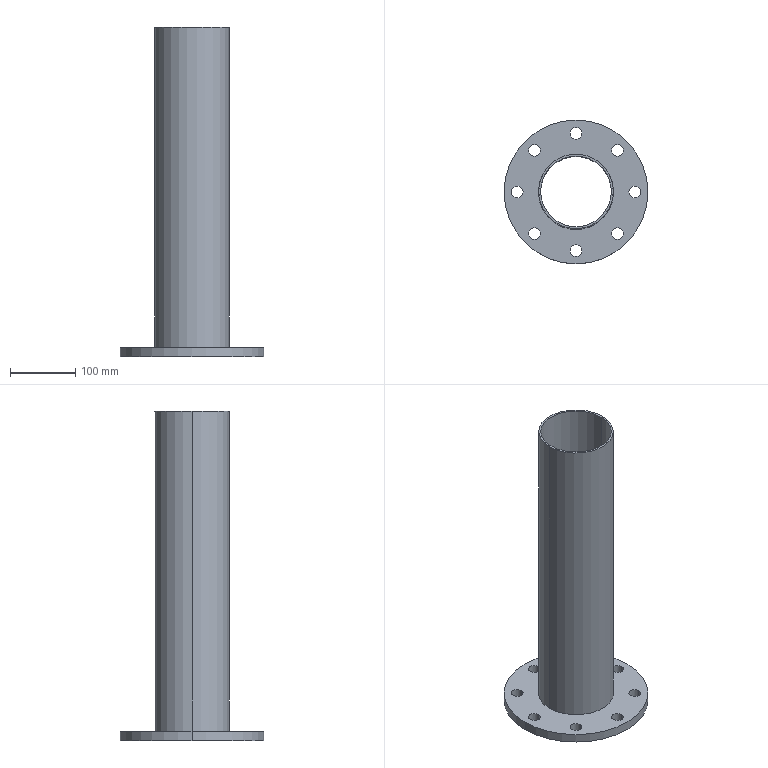Part | SolidWorks | features Extrusion 1, ICE 1 | 2 solids | 28 faces | box 220 x 220 x 504 mm | volume 882758 mm3 | cylinder 24 | plane 4 | commonest cylinder face diameters 18 x16 108.3 x2 114.3 x2 115 x2 220 x2
STEP:
#1=CARTESIAN_POINT('',(-72.64,63.64,14.));
#2=VERTEX_POINT('',#1);
#3=CARTESIAN_POINT('',(-54.64,63.64,14.));
#4=VERTEX_POINT('',#3);
#5=CARTESIAN_POINT('',(-63.64,63.64,14.));
#6=DIRECTION('',(0.,0.,1.));
#7=DIRECTION('',(1.,0.,0.));
#8=AXIS2_PLACEMENT_3D('',#5,#6,#7);
#9=CIRCLE('',#8,9.);
#10=EDGE_CURVE('',#2,#4,#9,.T.);
#11=ORIENTED_EDGE('',*,*,#10,.T.);
#12=CARTESIAN_POINT('',(-54.64,63.64,0.));
#13=VERTEX_POINT('',#12);
#14=CARTESIAN_POINT('',(-54.64,63.64,14.));
#15=DIRECTION('',(0.,0.,-1.));
#16=VECTOR('',#15,1000.);
#17=LINE('',#14,#16);
#18=EDGE_CURVE('',#4,#13,#17,.T.);
#19=ORIENTED_EDGE('',*,*,#18,.T.);
#20=CARTESIAN_POINT('',(-72.64,63.64,0.));
#21=VERTEX_POINT('',#20);
#22=CARTESIAN_POINT('',(-63.64,63.64,0.));
#23=DIRECTION('',(0.,0.,1.));
#24=DIRECTION('',(1.,0.,0.));
#25=AXIS2_PLACEMENT_3D('',#22,#23,#24);
#26=CIRCLE('',#25,9.);
#27=EDGE_CURVE('',#21,#13,#26,.T.);
#28=ORIENTED_EDGE('',*,*,#27,.F.);
#29=CARTESIAN_POINT('',(-72.64,63.64,14.));
#30=DIRECTION('',(0.,0.,-1.));
#31=VECTOR('',#30,1000.);
#32=LINE('',#29,#31);
#33=EDGE_CURVE('',#2,#21,#32,.T.);
#34=ORIENTED_EDGE('',*,*,#33,.F.);
#35=EDGE_LOOP('',(#11,#19,#28,#34));
#36=FACE_OUTER_BOUND('',#35,.T.);
#37=CARTESIAN_POINT('',(-63.64,63.64,14.));
#38=DIRECTION('',(0.,0.,-1.));
#39=DIRECTION('',(-1.,0.,0.));
#40=AXIS2_PLACEMENT_3D('',#37,#38,#39);
#41=CYLINDRICAL_SURFACE('',#40,9.);
#42=ADVANCED_FACE('',(#36),#41,.F.);
#43=CARTESIAN_POINT('',(-99.,0.,14.));
#44=VERTEX_POINT('',#43);
#45=CARTESIAN_POINT('',(-81.,0.,14.));
#46=VERTEX_POINT('',#45);
#47=CARTESIAN_POINT('',(-90.,0.,14.));
#48=DIRECTION('',(0.,0.,1.));
#49=DIRECTION('',(1.,0.,0.));
#50=AXIS2_PLACEMENT_3D('',#47,#48,#49);
#51=CIRCLE('',#50,9.);
#52=EDGE_CURVE('',#44,#46,#51,.T.);
#53=ORIENTED_EDGE('',*,*,#52,.T.);
#54=CARTESIAN_POINT('',(-81.,0.,0.));
#55=VERTEX_POINT('',#54);
#56=CARTESIAN_POINT('',(-81.,0.,14.));
#57=DIRECTION('',(0.,0.,-1.));
#58=VECTOR('',#57,1000.);
#59=LINE('',#56,#58);
#60=EDGE_CURVE('',#46,#55,#59,.T.);
#61=ORIENTED_EDGE('',*,*,#60,.T.);
#62=CARTESIAN_POINT('',(-99.,0.,0.));
#63=VERTEX_POINT('',#62);
#64=CARTESIAN_POINT('',(-90.,0.,0.));
#65=DIRECTION('',(0.,0.,1.));
#66=DIRECTION('',(1.,0.,0.));
#67=AXIS2_PLACEMENT_3D('',#64,#65,#66);
#68=CIRCLE('',#67,9.);
#69=EDGE_CURVE('',#63,#55,#68,.T.);
#70=ORIENTED_EDGE('',*,*,#69,.F.);
#71=CARTESIAN_POINT('',(-99.,0.,14.));
#72=DIRECTION('',(0.,0.,-1.));
#73=VECTOR('',#72,1000.);
#74=LINE('',#71,#73);
#75=EDGE_CURVE('',#44,#63,#74,.T.);
#76=ORIENTED_EDGE('',*,*,#75,.F.);
#77=EDGE_LOOP('',(#53,#61,#70,#76));
#78=FACE_OUTER_BOUND('',#77,.T.);
#79=CARTESIAN_POINT('',(-90.,0.,14.));
#80=DIRECTION('',(0.,0.,-1.));
#81=DIRECTION('',(-1.,0.,0.));
#82=AXIS2_PLACEMENT_3D('',#79,#80,#81);
#83=CYLINDRICAL_SURFACE('',#82,9.);
#84=ADVANCED_FACE('',(#78),#83,.F.);
#85=CARTESIAN_POINT('',(-72.64,-63.64,14.));
#86=VERTEX_POINT('',#85);
#87=CARTESIAN_POINT('',(-54.64,-63.64,14.));
#88=VERTEX_POINT('',#87);
#89=CARTESIAN_POINT('',(-63.64,-63.64,14.));
#90=DIRECTION('',(0.,0.,1.));
#91=DIRECTION('',(1.,0.,0.));
#92=AXIS2_PLACEMENT_3D('',#89,#90,#91);
#93=CIRCLE('',#92,9.);
#94=EDGE_CURVE('',#86,#88,#93,.T.);
#95=ORIENTED_EDGE('',*,*,#94,.T.);
#96=CARTESIAN_POINT('',(-54.64,-63.64,0.));
#97=VERTEX_POINT('',#96);
#98=CARTESIAN_POINT('',(-54.64,-63.64,14.));
#99=DIRECTION('',(0.,0.,-1.));
#100=VECTOR('',#99,1000.);
#101=LINE('',#98,#100);
#102=EDGE_CURVE('',#88,#97,#101,.T.);
#103=ORIENTED_EDGE('',*,*,#102,.T.);
#104=CARTESIAN_POINT('',(-72.64,-63.64,0.));
#105=VERTEX_POINT('',#104);
#106=CARTESIAN_POINT('',(-63.64,-63.64,0.));
#107=DIRECTION('',(0.,0.,1.));
#108=DIRECTION('',(1.,0.,0.));
#109=AXIS2_PLACEMENT_3D('',#106,#107,#108);
#110=CIRCLE('',#109,9.);
#111=EDGE_CURVE('',#105,#97,#110,.T.);
#112=ORIENTED_EDGE('',*,*,#111,.F.);
#113=CARTESIAN_POINT('',(-72.64,-63.64,14.));
#114=DIRECTION('',(0.,0.,-1.));
#115=VECTOR('',#114,1000.);
#116=LINE('',#113,#115);
#117=EDGE_CURVE('',#86,#105,#116,.T.);
#118=ORIENTED_EDGE('',*,*,#117,.F.);
#119=EDGE_LOOP('',(#95,#103,#112,#118));
#120=FACE_OUTER_BOUND('',#119,.T.);
#121=CARTESIAN_POINT('',(-63.64,-63.64,14.));
#122=DIRECTION('',(0.,0.,-1.));
#123=DIRECTION('',(-1.,0.,0.));
#124=AXIS2_PLACEMENT_3D('',#121,#122,#123);
#125=CYLINDRICAL_SURFACE('',#124,9.);
#126=ADVANCED_FACE('',(#120),#125,.F.);
#127=CARTESIAN_POINT('',(-9.,-90.,14.));
#128=VERTEX_POINT('',#127);
#129=CARTESIAN_POINT('',(9.,-90.,14.));
#130=VERTEX_POINT('',#129);
#131=CARTESIAN_POINT('',(0.,-90.,14.));
#132=DIRECTION('',(0.,0.,1.));
#133=DIRECTION('',(1.,0.,0.));
#134=AXIS2_PLACEMENT_3D('',#131,#132,#133);
#135=CIRCLE('',#134,9.);
#136=EDGE_CURVE('',#128,#130,#135,.T.);
#137=ORIENTED_EDGE('',*,*,#136,.T.);
#138=CARTESIAN_POINT('',(9.,-90.,0.));
#139=VERTEX_POINT('',#138);
#140=CARTESIAN_POINT('',(9.,-90.,14.));
#141=DIRECTION('',(0.,0.,-1.));
#142=VECTOR('',#141,1000.);
#143=LINE('',#140,#142);
#144=EDGE_CURVE('',#130,#139,#143,.T.);
#145=ORIENTED_EDGE('',*,*,#144,.T.);
#146=CARTESIAN_POINT('',(-9.,-90.,0.));
#147=VERTEX_POINT('',#146);
#148=CARTESIAN_POINT('',(0.,-90.,0.));
#149=DIRECTION('',(0.,0.,1.));
#150=DIRECTION('',(1.,0.,0.));
#151=AXIS2_PLACEMENT_3D('',#148,#149,#150);
#152=CIRCLE('',#151,9.);
#153=EDGE_CURVE('',#147,#139,#152,.T.);
#154=ORIENTED_EDGE('',*,*,#153,.F.);
#155=CARTESIAN_POINT('',(-9.,-90.,14.));
#156=DIRECTION('',(0.,0.,-1.));
#157=VECTOR('',#156,1000.);
#158=LINE('',#155,#157);
#159=EDGE_CURVE('',#128,#147,#158,.T.);
#160=ORIENTED_EDGE('',*,*,#159,.F.);
#161=EDGE_LOOP('',(#137,#145,#154,#160));
#162=FACE_OUTER_BOUND('',#161,.T.);
#163=CARTESIAN_POINT('',(0.,-90.,14.));
#164=DIRECTION('',(0.,0.,-1.));
#165=DIRECTION('',(-1.,0.,0.));
#166=AXIS2_PLACEMENT_3D('',#163,#164,#165);
#167=CYLINDRICAL_SURFACE('',#166,9.);
#168=ADVANCED_FACE('',(#162),#167,.F.);
#169=CARTESIAN_POINT('',(54.64,-63.64,14.));
#170=VERTEX_POINT('',#169);
#171=CARTESIAN_POINT('',(72.64,-63.64,14.));
#172=VERTEX_POINT('',#171);
#173=CARTESIAN_POINT('',(63.64,-63.64,14.));
#174=DIRECTION('',(0.,0.,1.));
#175=DIRECTION('',(1.,0.,0.));
#176=AXIS2_PLACEMENT_3D('',#173,#174,#175);
#177=CIRCLE('',#176,9.);
#178=EDGE_CURVE('',#170,#172,#177,.T.);
#179=ORIENTED_EDGE('',*,*,#178,.T.);
#180=CARTESIAN_POINT('',(72.64,-63.64,0.));
#181=VERTEX_POINT('',#180);
#182=CARTESIAN_POINT('',(72.64,-63.64,14.));
#183=DIRECTION('',(0.,0.,-1.));
#184=VECTOR('',#183,1000.);
#185=LINE('',#182,#184);
#186=EDGE_CURVE('',#172,#181,#185,.T.);
#187=ORIENTED_EDGE('',*,*,#186,.T.);
#188=CARTESIAN_POINT('',(54.64,-63.64,0.));
#189=VERTEX_POINT('',#188);
#190=CARTESIAN_POINT('',(63.64,-63.64,0.));
#191=DIRECTION('',(0.,0.,1.));
#192=DIRECTION('',(1.,0.,0.));
#193=AXIS2_PLACEMENT_3D('',#190,#191,#192);
#194=CIRCLE('',#193,9.);
#195=EDGE_CURVE('',#189,#181,#194,.T.);
#196=ORIENTED_EDGE('',*,*,#195,.F.);
#197=CARTESIAN_POINT('',(54.64,-63.64,14.));
#198=DIRECTION('',(0.,0.,-1.));
#199=VECTOR('',#198,1000.);
#200=LINE('',#197,#199);
#201=EDGE_CURVE('',#170,#189,#200,.T.);
#202=ORIENTED_EDGE('',*,*,#201,.F.);
#203=EDGE_LOOP('',(#179,#187,#196,#202));
#204=FACE_OUTER_BOUND('',#203,.T.);
#205=CARTESIAN_POINT('',(63.64,-63.64,14.));
#206=DIRECTION('',(0.,0.,-1.));
#207=DIRECTION('',(-1.,0.,0.));
#208=AXIS2_PLACEMENT_3D('',#205,#206,#207);
#209=CYLINDRICAL_SURFACE('',#208,9.);
#210=ADVANCED_FACE('',(#204),#209,.F.);
#211=CARTESIAN_POINT('',(81.,0.,14.));
#212=VERTEX_POINT('',#211);
#213=CARTESIAN_POINT('',(99.,0.,14.));
#214=VERTEX_POINT('',#213);
#215=CARTESIAN_POINT('',(90.,0.,14.));
#216=DIRECTION('',(0.,0.,1.));
#217=DIRECTION('',(1.,0.,0.));
#218=AXIS2_PLACEMENT_3D('',#215,#216,#217);
#219=CIRCLE('',#218,9.);
#220=EDGE_CURVE('',#212,#214,#219,.T.);
#221=ORIENTED_EDGE('',*,*,#220,.T.);
#222=CARTESIAN_POINT('',(99.,0.,0.));
#223=VERTEX_POINT('',#222);
#224=CARTESIAN_POINT('',(99.,0.,14.));
#225=DIRECTION('',(0.,0.,-1.));
#226=VECTOR('',#225,1000.);
#227=LINE('',#224,#226);
#228=EDGE_CURVE('',#214,#223,#227,.T.);
#229=ORIENTED_EDGE('',*,*,#228,.T.);
#230=CARTESIAN_POINT('',(81.,0.,0.));
#231=VERTEX_POINT('',#230);
#232=CARTESIAN_POINT('',(90.,0.,0.));
#233=DIRECTION('',(0.,0.,1.));
#234=DIRECTION('',(1.,0.,0.));
#235=AXIS2_PLACEMENT_3D('',#232,#233,#234);
#236=CIRCLE('',#235,9.);
#237=EDGE_CURVE('',#231,#223,#236,.T.);
#238=ORIENTED_EDGE('',*,*,#237,.F.);
#239=CARTESIAN_POINT('',(81.,0.,14.));
#240=DIRECTION('',(0.,0.,-1.));
#241=VECTOR('',#240,1000.);
#242=LINE('',#239,#241);
#243=EDGE_CURVE('',#212,#231,#242,.T.);
#244=ORIENTED_EDGE('',*,*,#243,.F.);
#245=EDGE_LOOP('',(#221,#229,#238,#244));
#246=FACE_OUTER_BOUND('',#245,.T.);
#247=CARTESIAN_POINT('',(90.,0.,14.));
#248=DIRECTION('',(0.,0.,-1.));
#249=DIRECTION('',(-1.,0.,0.));
#250=AXIS2_PLACEMENT_3D('',#247,#248,#249);
#251=CYLINDRICAL_SURFACE('',#250,9.);
#252=ADVANCED_FACE('',(#246),#251,.F.);
#253=CARTESIAN_POINT('',(54.64,63.64,14.));
#254=VERTEX_POINT('',#253);
#255=CARTESIAN_POINT('',(72.64,63.64,14.));
#256=VERTEX_POINT('',#255);
#257=CARTESIAN_POINT('',(63.64,63.64,14.));
#258=DIRECTION('',(0.,0.,1.));
#259=DIRECTION('',(1.,0.,0.));
#260=AXIS2_PLACEMENT_3D('',#257,#258,#259);
#261=CIRCLE('',#260,9.);
#262=EDGE_CURVE('',#254,#256,#261,.T.);
#263=ORIENTED_EDGE('',*,*,#262,.T.);
#264=CARTESIAN_POINT('',(72.64,63.64,0.));
#265=VERTEX_POINT('',#264);
#266=CARTESIAN_POINT('',(72.64,63.64,14.));
#267=DIRECTION('',(0.,0.,-1.));
#268=VECTOR('',#267,1000.);
#269=LINE('',#266,#268);
#270=EDGE_CURVE('',#256,#265,#269,.T.);
#271=ORIENTED_EDGE('',*,*,#270,.T.);
#272=CARTESIAN_POINT('',(54.64,63.64,0.));
#273=VERTEX_POINT('',#272);
#274=CARTESIAN_POINT('',(63.64,63.64,0.));
#275=DIRECTION('',(0.,0.,1.));
#276=DIRECTION('',(1.,0.,0.));
#277=AXIS2_PLACEMENT_3D('',#274,#275,#276);
#278=CIRCLE('',#277,9.);
#279=EDGE_CURVE('',#273,#265,#278,.T.);
#280=ORIENTED_EDGE('',*,*,#279,.F.);
#281=CARTESIAN_POINT('',(54.64,63.64,14.));
#282=DIRECTION('',(0.,0.,-1.));
#283=VECTOR('',#282,1000.);
#284=LINE('',#281,#283);
#285=EDGE_CURVE('',#254,#273,#284,.T.);
#286=ORIENTED_EDGE('',*,*,#285,.F.);
#287=EDGE_LOOP('',(#263,#271,#280,#286));
#288=FACE_OUTER_BOUND('',#287,.T.);
#289=CARTESIAN_POINT('',(63.64,63.64,14.));
#290=DIRECTION('',(0.,0.,-1.));
#291=DIRECTION('',(-1.,0.,0.));
#292=AXIS2_PLACEMENT_3D('',#289,#290,#291);
#293=CYLINDRICAL_SURFACE('',#292,9.);
#294=ADVANCED_FACE('',(#288),#293,.F.);
#295=CARTESIAN_POINT('',(-9.,90.,14.));
#296=VERTEX_POINT('',#295);
#297=CARTESIAN_POINT('',(9.,90.,14.));
#298=VERTEX_POINT('',#297);
#299=CARTESIAN_POINT('',(0.,90.,14.));
#300=DIRECTION('',(0.,0.,1.));
#301=DIRECTION('',(1.,0.,0.));
#302=AXIS2_PLACEMENT_3D('',#299,#300,#301);
#303=CIRCLE('',#302,9.);
#304=EDGE_CURVE('',#296,#298,#303,.T.);
#305=ORIENTED_EDGE('',*,*,#304,.T.);
#306=CARTESIAN_POINT('',(9.,90.,0.));
#307=VERTEX_POINT('',#306);
#308=CARTESIAN_POINT('',(9.,90.,14.));
#309=DIRECTION('',(0.,0.,-1.));
#310=VECTOR('',#309,1000.);
#311=LINE('',#308,#310);
#312=EDGE_CURVE('',#298,#307,#311,.T.);
#313=ORIENTED_EDGE('',*,*,#312,.T.);
#314=CARTESIAN_POINT('',(-9.,90.,0.));
#315=VERTEX_POINT('',#314);
#316=CARTESIAN_POINT('',(0.,90.,0.));
#317=DIRECTION('',(0.,0.,1.));
#318=DIRECTION('',(1.,0.,0.));
#319=AXIS2_PLACEMENT_3D('',#316,#317,#318);
#320=CIRCLE('',#319,9.);
#321=EDGE_CURVE('',#315,#307,#320,.T.);
#322=ORIENTED_EDGE('',*,*,#321,.F.);
#323=CARTESIAN_POINT('',(-9.,90.,14.));
#324=DIRECTION('',(0.,0.,-1.));
#325=VECTOR('',#324,1000.);
#326=LINE('',#323,#325);
#327=EDGE_CURVE('',#296,#315,#326,.T.);
#328=ORIENTED_EDGE('',*,*,#327,.F.);
#329=EDGE_LOOP('',(#305,#313,#322,#328));
#330=FACE_OUTER_BOUND('',#329,.T.);
#331=CARTESIAN_POINT('',(0.,90.,14.));
#332=DIRECTION('',(0.,0.,-1.));
#333=DIRECTION('',(-1.,0.,0.));
#334=AXIS2_PLACEMENT_3D('',#331,#332,#333);
#335=CYLINDRICAL_SURFACE('',#334,9.);
#336=ADVANCED_FACE('',(#330),#335,.F.);
#337=CARTESIAN_POINT('',(-57.5,0.,14.));
#338=VERTEX_POINT('',#337);
#339=CARTESIAN_POINT('',(57.5,0.,14.));
#340=VERTEX_POINT('',#339);
#341=CARTESIAN_POINT('',(0.,0.,14.));
#342=DIRECTION('',(0.,0.,1.));
#343=DIRECTION('',(1.,0.,0.));
#344=AXIS2_PLACEMENT_3D('',#341,#342,#343);
#345=CIRCLE('',#344,57.5);
#346=EDGE_CURVE('',#338,#340,#345,.T.);
#347=ORIENTED_EDGE('',*,*,#346,.T.);
#348=CARTESIAN_POINT('',(57.5,0.,0.));
#349=VERTEX_POINT('',#348);
#350=CARTESIAN_POINT('',(57.5,0.,14.));
#351=DIRECTION('',(0.,0.,-1.));
#352=VECTOR('',#351,1000.);
#353=LINE('',#350,#352);
#354=EDGE_CURVE('',#340,#349,#353,.T.);
#355=ORIENTED_EDGE('',*,*,#354,.T.);
#356=CARTESIAN_POINT('',(-57.5,0.,0.));
#357=VERTEX_POINT('',#356);
#358=CARTESIAN_POINT('',(0.,0.,0.));
#359=DIRECTION('',(0.,0.,1.));
#360=DIRECTION('',(1.,0.,0.));
#361=AXIS2_PLACEMENT_3D('',#358,#359,#360);
#362=CIRCLE('',#361,57.5);
#363=EDGE_CURVE('',#357,#349,#362,.T.);
#364=ORIENTED_EDGE('',*,*,#363,.F.);
#365=CARTESIAN_POINT('',(-57.5,0.,14.));
#366=DIRECTION('',(0.,0.,-1.));
#367=VECTOR('',#366,1000.);
#368=LINE('',#365,#367);
#369=EDGE_CURVE('',#338,#357,#368,.T.);
#370=ORIENTED_EDGE('',*,*,#369,.F.);
#371=EDGE_LOOP('',(#347,#355,#364,#370));
#372=FACE_OUTER_BOUND('',#371,.T.);
#373=CARTESIAN_POINT('',(0.,0.,14.));
#374=DIRECTION('',(0.,0.,-1.));
#375=DIRECTION('',(-1.,0.,0.));
#376=AXIS2_PLACEMENT_3D('',#373,#374,#375);
#377=CYLINDRICAL_SURFACE('',#376,57.5);
#378=ADVANCED_FACE('',(#372),#377,.F.);
#379=CARTESIAN_POINT('',(110.,0.,14.));
#380=VERTEX_POINT('',#379);
#381=CARTESIAN_POINT('',(-110.,0.,14.));
#382=VERTEX_POINT('',#381);
#383=CARTESIAN_POINT('',(0.,0.,14.));
#384=DIRECTION('',(0.,0.,1.));
#385=DIRECTION('',(1.,0.,0.));
#386=AXIS2_PLACEMENT_3D('',#383,#384,#385);
#387=CIRCLE('',#386,110.);
#388=EDGE_CURVE('',#380,#382,#387,.T.);
#389=ORIENTED_EDGE('',*,*,#388,.F.);
#390=CARTESIAN_POINT('',(110.,0.,0.));
#391=VERTEX_POINT('',#390);
#392=CARTESIAN_POINT('',(110.,0.,14.));
#393=DIRECTION('',(0.,0.,-1.));
#394=VECTOR('',#393,1000.);
#395=LINE('',#392,#394);
#396=EDGE_CURVE('',#380,#391,#395,.T.);
#397=ORIENTED_EDGE('',*,*,#396,.T.);
#398=CARTESIAN_POINT('',(-110.,0.,0.));
#399=VERTEX_POINT('',#398);
#400=CARTESIAN_POINT('',(0.,0.,0.));
#401=DIRECTION('',(0.,0.,1.));
#402=DIRECTION('',(1.,0.,0.));
#403=AXIS2_PLACEMENT_3D('',#400,#401,#402);
#404=CIRCLE('',#403,110.);
#405=EDGE_CURVE('',#391,#399,#404,.T.);
#406=ORIENTED_EDGE('',*,*,#405,.T.);
#407=CARTESIAN_POINT('',(-110.,0.,14.));
#408=DIRECTION('',(0.,0.,-1.));
#409=VECTOR('',#408,1000.);
#410=LINE('',#407,#409);
#411=EDGE_CURVE('',#382,#399,#410,.T.);
#412=ORIENTED_EDGE('',*,*,#411,.F.);
#413=EDGE_LOOP('',(#389,#397,#406,#412));
#414=FACE_OUTER_BOUND('',#413,.T.);
#415=CARTESIAN_POINT('',(0.,0.,14.));
#416=DIRECTION('',(0.,0.,-1.));
#417=DIRECTION('',(-1.,0.,0.));
#418=AXIS2_PLACEMENT_3D('',#415,#416,#417);
#419=CYLINDRICAL_SURFACE('',#418,110.);
#420=ADVANCED_FACE('',(#414),#419,.T.);
#421=ORIENTED_EDGE('',*,*,#52,.F.);
#422=CARTESIAN_POINT('',(-90.,0.,14.));
#423=DIRECTION('',(0.,0.,1.));
#424=DIRECTION('',(1.,0.,0.));
#425=AXIS2_PLACEMENT_3D('',#422,#423,#424);
#426=CIRCLE('',#425,9.);
#427=EDGE_CURVE('',#46,#44,#426,.T.);
#428=ORIENTED_EDGE('',*,*,#427,.F.);
#429=EDGE_LOOP('',(#421,#428));
#430=FACE_BOUND('',#429,.T.);
#431=ORIENTED_EDGE('',*,*,#136,.F.);
#432=CARTESIAN_POINT('',(0.,-90.,14.));
#433=DIRECTION('',(0.,0.,1.));
#434=DIRECTION('',(1.,0.,0.));
#435=AXIS2_PLACEMENT_3D('',#432,#433,#434);
#436=CIRCLE('',#435,9.);
#437=EDGE_CURVE('',#130,#128,#436,.T.);
#438=ORIENTED_EDGE('',*,*,#437,.F.);
#439=EDGE_LOOP('',(#431,#438));
#440=FACE_BOUND('',#439,.T.);
#441=ORIENTED_EDGE('',*,*,#220,.F.);
#442=CARTESIAN_POINT('',(90.,0.,14.));
#443=DIRECTION('',(0.,0.,1.));
#444=DIRECTION('',(1.,0.,0.));
#445=AXIS2_PLACEMENT_3D('',#442,#443,#444);
#446=CIRCLE('',#445,9.);
#447=EDGE_CURVE('',#214,#212,#446,.T.);
#448=ORIENTED_EDGE('',*,*,#447,.F.);
#449=EDGE_LOOP('',(#441,#448));
#450=FACE_BOUND('',#449,.T.);
#451=ORIENTED_EDGE('',*,*,#304,.F.);
#452=CARTESIAN_POINT('',(0.,90.,14.));
#453=DIRECTION('',(0.,0.,1.));
#454=DIRECTION('',(1.,0.,0.));
#455=AXIS2_PLACEMENT_3D('',#452,#453,#454);
#456=CIRCLE('',#455,9.);
#457=EDGE_CURVE('',#298,#296,#456,.T.);
#458=ORIENTED_EDGE('',*,*,#457,.F.);
#459=EDGE_LOOP('',(#451,#458));
#460=FACE_BOUND('',#459,.T.);
#461=CARTESIAN_POINT('',(0.,0.,14.));
#462=DIRECTION('',(0.,0.,1.));
#463=DIRECTION('',(1.,0.,0.));
#464=AXIS2_PLACEMENT_3D('',#461,#462,#463);
#465=CIRCLE('',#464,110.);
#466=EDGE_CURVE('',#382,#380,#465,.T.);
#467=ORIENTED_EDGE('',*,*,#466,.T.);
#468=ORIENTED_EDGE('',*,*,#388,.T.);
#469=EDGE_LOOP('',(#467,#468));
#470=FACE_OUTER_BOUND('',#469,.T.);
#471=ORIENTED_EDGE('',*,*,#346,.F.);
#472=CARTESIAN_POINT('',(0.,0.,14.));
#473=DIRECTION('',(0.,0.,1.));
#474=DIRECTION('',(1.,0.,0.));
#475=AXIS2_PLACEMENT_3D('',#472,#473,#474);
#476=CIRCLE('',#475,57.5);
#477=EDGE_CURVE('',#340,#338,#476,.T.);
#478=ORIENTED_EDGE('',*,*,#477,.F.);
#479=EDGE_LOOP('',(#471,#478));
#480=FACE_BOUND('',#479,.T.);
#481=ORIENTED_EDGE('',*,*,#262,.F.);
#482=CARTESIAN_POINT('',(63.64,63.64,14.));
#483=DIRECTION('',(0.,0.,1.));
#484=DIRECTION('',(1.,0.,0.));
#485=AXIS2_PLACEMENT_3D('',#482,#483,#484);
#486=CIRCLE('',#485,9.);
#487=EDGE_CURVE('',#256,#254,#486,.T.);
#488=ORIENTED_EDGE('',*,*,#487,.F.);
#489=EDGE_LOOP('',(#481,#488));
#490=FACE_BOUND('',#489,.T.);
#491=ORIENTED_EDGE('',*,*,#178,.F.);
#492=CARTESIAN_POINT('',(63.64,-63.64,14.));
#493=DIRECTION('',(0.,0.,1.));
#494=DIRECTION('',(1.,0.,0.));
#495=AXIS2_PLACEMENT_3D('',#492,#493,#494);
#496=CIRCLE('',#495,9.);
#497=EDGE_CURVE('',#172,#170,#496,.T.);
#498=ORIENTED_EDGE('',*,*,#497,.F.);
#499=EDGE_LOOP('',(#491,#498));
#500=FACE_BOUND('',#499,.T.);
#501=ORIENTED_EDGE('',*,*,#94,.F.);
#502=CARTESIAN_POINT('',(-63.64,-63.64,14.));
#503=DIRECTION('',(0.,0.,1.));
#504=DIRECTION('',(1.,0.,0.));
#505=AXIS2_PLACEMENT_3D('',#502,#503,#504);
#506=CIRCLE('',#505,9.);
#507=EDGE_CURVE('',#88,#86,#506,.T.);
#508=ORIENTED_EDGE('',*,*,#507,.F.);
#509=EDGE_LOOP('',(#501,#508));
#510=FACE_BOUND('',#509,.T.);
#511=ORIENTED_EDGE('',*,*,#10,.F.);
#512=CARTESIAN_POINT('',(-63.64,63.64,14.));
#513=DIRECTION('',(0.,0.,1.));
#514=DIRECTION('',(1.,0.,0.));
#515=AXIS2_PLACEMENT_3D('',#512,#513,#514);
#516=CIRCLE('',#515,9.);
#517=EDGE_CURVE('',#4,#2,#516,.T.);
#518=ORIENTED_EDGE('',*,*,#517,.F.);
#519=EDGE_LOOP('',(#511,#518));
#520=FACE_BOUND('',#519,.T.);
#521=CARTESIAN_POINT('',(0.,0.,14.));
#522=DIRECTION('',(0.,0.,1.));
#523=DIRECTION('',(1.,0.,0.));
#524=AXIS2_PLACEMENT_3D('',#521,#522,#523);
#525=PLANE('',#524);
#526=ADVANCED_FACE('',(#430,#440,#450,#460,#470,#480,#490,#500,#510,#520),#525,.T.);
#527=CARTESIAN_POINT('',(0.,0.,0.));
#528=DIRECTION('',(0.,0.,1.));
#529=DIRECTION('',(1.,0.,0.));
#530=AXIS2_PLACEMENT_3D('',#527,#528,#529);
#531=CIRCLE('',#530,110.);
#532=EDGE_CURVE('',#399,#391,#531,.T.);
#533=ORIENTED_EDGE('',*,*,#532,.F.);
#534=ORIENTED_EDGE('',*,*,#405,.F.);
#535=EDGE_LOOP('',(#533,#534));
#536=FACE_OUTER_BOUND('',#535,.T.);
#537=ORIENTED_EDGE('',*,*,#363,.T.);
#538=CARTESIAN_POINT('',(0.,0.,0.));
#539=DIRECTION('',(0.,0.,1.));
#540=DIRECTION('',(1.,0.,0.));
#541=AXIS2_PLACEMENT_3D('',#538,#539,#540);
#542=CIRCLE('',#541,57.5);
#543=EDGE_CURVE('',#349,#357,#542,.T.);
#544=ORIENTED_EDGE('',*,*,#543,.T.);
#545=EDGE_LOOP('',(#537,#544));
#546=FACE_BOUND('',#545,.T.);
#547=ORIENTED_EDGE('',*,*,#321,.T.);
#548=CARTESIAN_POINT('',(0.,90.,0.));
#549=DIRECTION('',(0.,0.,1.));
#550=DIRECTION('',(1.,0.,0.));
#551=AXIS2_PLACEMENT_3D('',#548,#549,#550);
#552=CIRCLE('',#551,9.);
#553=EDGE_CURVE('',#307,#315,#552,.T.);
#554=ORIENTED_EDGE('',*,*,#553,.T.);
#555=EDGE_LOOP('',(#547,#554));
#556=FACE_BOUND('',#555,.T.);
#557=ORIENTED_EDGE('',*,*,#279,.T.);
#558=CARTESIAN_POINT('',(63.64,63.64,0.));
#559=DIRECTION('',(0.,0.,1.));
#560=DIRECTION('',(1.,0.,0.));
#561=AXIS2_PLACEMENT_3D('',#558,#559,#560);
#562=CIRCLE('',#561,9.);
#563=EDGE_CURVE('',#265,#273,#562,.T.);
#564=ORIENTED_EDGE('',*,*,#563,.T.);
#565=EDGE_LOOP('',(#557,#564));
#566=FACE_BOUND('',#565,.T.);
#567=ORIENTED_EDGE('',*,*,#237,.T.);
#568=CARTESIAN_POINT('',(90.,0.,0.));
#569=DIRECTION('',(0.,0.,1.));
#570=DIRECTION('',(1.,0.,0.));
#571=AXIS2_PLACEMENT_3D('',#568,#569,#570);
#572=CIRCLE('',#571,9.);
#573=EDGE_CURVE('',#223,#231,#572,.T.);
#574=ORIENTED_EDGE('',*,*,#573,.T.);
#575=EDGE_LOOP('',(#567,#574));
#576=FACE_BOUND('',#575,.T.);
#577=ORIENTED_EDGE('',*,*,#195,.T.);
#578=CARTESIAN_POINT('',(63.64,-63.64,0.));
#579=DIRECTION('',(0.,0.,1.));
#580=DIRECTION('',(1.,0.,0.));
#581=AXIS2_PLACEMENT_3D('',#578,#579,#580);
#582=CIRCLE('',#581,9.);
#583=EDGE_CURVE('',#181,#189,#582,.T.);
#584=ORIENTED_EDGE('',*,*,#583,.T.);
#585=EDGE_LOOP('',(#577,#584));
#586=FACE_BOUND('',#585,.T.);
#587=ORIENTED_EDGE('',*,*,#153,.T.);
#588=CARTESIAN_POINT('',(0.,-90.,0.));
#589=DIRECTION('',(0.,0.,1.));
#590=DIRECTION('',(1.,0.,0.));
#591=AXIS2_PLACEMENT_3D('',#588,#589,#590);
#592=CIRCLE('',#591,9.);
#593=EDGE_CURVE('',#139,#147,#592,.T.);
#594=ORIENTED_EDGE('',*,*,#593,.T.);
#595=EDGE_LOOP('',(#587,#594));
#596=FACE_BOUND('',#595,.T.);
#597=ORIENTED_EDGE('',*,*,#111,.T.);
#598=CARTESIAN_POINT('',(-63.64,-63.64,0.));
#599=DIRECTION('',(0.,0.,1.));
#600=DIRECTION('',(1.,0.,0.));
#601=AXIS2_PLACEMENT_3D('',#598,#599,#600);
#602=CIRCLE('',#601,9.);
#603=EDGE_CURVE('',#97,#105,#602,.T.);
#604=ORIENTED_EDGE('',*,*,#603,.T.);
#605=EDGE_LOOP('',(#597,#604));
#606=FACE_BOUND('',#605,.T.);
#607=ORIENTED_EDGE('',*,*,#69,.T.);
#608=CARTESIAN_POINT('',(-90.,0.,0.));
#609=DIRECTION('',(0.,0.,1.));
#610=DIRECTION('',(1.,0.,0.));
#611=AXIS2_PLACEMENT_3D('',#608,#609,#610);
#612=CIRCLE('',#611,9.);
#613=EDGE_CURVE('',#55,#63,#612,.T.);
#614=ORIENTED_EDGE('',*,*,#613,.T.);
#615=EDGE_LOOP('',(#607,#614));
#616=FACE_BOUND('',#615,.T.);
#617=ORIENTED_EDGE('',*,*,#27,.T.);
#618=CARTESIAN_POINT('',(-63.64,63.64,0.));
#619=DIRECTION('',(0.,0.,1.));
#620=DIRECTION('',(1.,0.,0.));
#621=AXIS2_PLACEMENT_3D('',#618,#619,#620);
#622=CIRCLE('',#621,9.);
#623=EDGE_CURVE('',#13,#21,#622,.T.);
#624=ORIENTED_EDGE('',*,*,#623,.T.);
#625=EDGE_LOOP('',(#617,#624));
#626=FACE_BOUND('',#625,.T.);
#627=CARTESIAN_POINT('',(0.,0.,0.));
#628=DIRECTION('',(0.,0.,1.));
#629=DIRECTION('',(1.,0.,0.));
#630=AXIS2_PLACEMENT_3D('',#627,#628,#629);
#631=PLANE('',#630);
#632=ADVANCED_FACE('',(#536,#546,#556,#566,#576,#586,#596,#606,#616,#626),#631,.F.);
#633=ORIENTED_EDGE('',*,*,#396,.F.);
#634=ORIENTED_EDGE('',*,*,#466,.F.);
#635=ORIENTED_EDGE('',*,*,#411,.T.);
#636=ORIENTED_EDGE('',*,*,#532,.T.);
#637=EDGE_LOOP('',(#633,#634,#635,#636));
#638=FACE_OUTER_BOUND('',#637,.T.);
#639=CARTESIAN_POINT('',(0.,0.,14.));
#640=DIRECTION('',(0.,0.,-1.));
#641=DIRECTION('',(-1.,0.,0.));
#642=AXIS2_PLACEMENT_3D('',#639,#640,#641);
#643=CYLINDRICAL_SURFACE('',#642,110.);
#644=ADVANCED_FACE('',(#638),#643,.T.);
#645=ORIENTED_EDGE('',*,*,#354,.F.);
#646=ORIENTED_EDGE('',*,*,#477,.T.);
#647=ORIENTED_EDGE('',*,*,#369,.T.);
#648=ORIENTED_EDGE('',*,*,#543,.F.);
#649=EDGE_LOOP('',(#645,#646,#647,#648));
#650=FACE_OUTER_BOUND('',#649,.T.);
#651=CARTESIAN_POINT('',(0.,0.,14.));
#652=DIRECTION('',(0.,0.,-1.));
#653=DIRECTION('',(-1.,0.,0.));
#654=AXIS2_PLACEMENT_3D('',#651,#652,#653);
#655=CYLINDRICAL_SURFACE('',#654,57.5);
#656=ADVANCED_FACE('',(#650),#655,.F.);
#657=ORIENTED_EDGE('',*,*,#312,.F.);
#658=ORIENTED_EDGE('',*,*,#457,.T.);
#659=ORIENTED_EDGE('',*,*,#327,.T.);
#660=ORIENTED_EDGE('',*,*,#553,.F.);
#661=EDGE_LOOP('',(#657,#658,#659,#660));
#662=FACE_OUTER_BOUND('',#661,.T.);
#663=CARTESIAN_POINT('',(0.,90.,14.));
#664=DIRECTION('',(0.,0.,-1.));
#665=DIRECTION('',(-1.,0.,0.));
#666=AXIS2_PLACEMENT_3D('',#663,#664,#665);
#667=CYLINDRICAL_SURFACE('',#666,9.);
#668=ADVANCED_FACE('',(#662),#667,.F.);
#669=ORIENTED_EDGE('',*,*,#270,.F.);
#670=ORIENTED_EDGE('',*,*,#487,.T.);
#671=ORIENTED_EDGE('',*,*,#285,.T.);
#672=ORIENTED_EDGE('',*,*,#563,.F.);
#673=EDGE_LOOP('',(#669,#670,#671,#672));
#674=FACE_OUTER_BOUND('',#673,.T.);
#675=CARTESIAN_POINT('',(63.64,63.64,14.));
#676=DIRECTION('',(0.,0.,-1.));
#677=DIRECTION('',(-1.,0.,0.));
#678=AXIS2_PLACEMENT_3D('',#675,#676,#677);
#679=CYLINDRICAL_SURFACE('',#678,9.);
#680=ADVANCED_FACE('',(#674),#679,.F.);
#681=ORIENTED_EDGE('',*,*,#228,.F.);
#682=ORIENTED_EDGE('',*,*,#447,.T.);
#683=ORIENTED_EDGE('',*,*,#243,.T.);
#684=ORIENTED_EDGE('',*,*,#573,.F.);
#685=EDGE_LOOP('',(#681,#682,#683,#684));
#686=FACE_OUTER_BOUND('',#685,.T.);
#687=CARTESIAN_POINT('',(90.,0.,14.));
#688=DIRECTION('',(0.,0.,-1.));
#689=DIRECTION('',(-1.,0.,0.));
#690=AXIS2_PLACEMENT_3D('',#687,#688,#689);
#691=CYLINDRICAL_SURFACE('',#690,9.);
#692=ADVANCED_FACE('',(#686),#691,.F.);
#693=ORIENTED_EDGE('',*,*,#186,.F.);
#694=ORIENTED_EDGE('',*,*,#497,.T.);
#695=ORIENTED_EDGE('',*,*,#201,.T.);
#696=ORIENTED_EDGE('',*,*,#583,.F.);
#697=EDGE_LOOP('',(#693,#694,#695,#696));
#698=FACE_OUTER_BOUND('',#697,.T.);
#699=CARTESIAN_POINT('',(63.64,-63.64,14.));
#700=DIRECTION('',(0.,0.,-1.));
#701=DIRECTION('',(-1.,0.,0.));
#702=AXIS2_PLACEMENT_3D('',#699,#700,#701);
#703=CYLINDRICAL_SURFACE('',#702,9.);
#704=ADVANCED_FACE('',(#698),#703,.F.);
#705=ORIENTED_EDGE('',*,*,#144,.F.);
#706=ORIENTED_EDGE('',*,*,#437,.T.);
#707=ORIENTED_EDGE('',*,*,#159,.T.);
#708=ORIENTED_EDGE('',*,*,#593,.F.);
#709=EDGE_LOOP('',(#705,#706,#707,#708));
#710=FACE_OUTER_BOUND('',#709,.T.);
#711=CARTESIAN_POINT('',(0.,-90.,14.));
#712=DIRECTION('',(0.,0.,-1.));
#713=DIRECTION('',(-1.,0.,0.));
#714=AXIS2_PLACEMENT_3D('',#711,#712,#713);
#715=CYLINDRICAL_SURFACE('',#714,9.);
#716=ADVANCED_FACE('',(#710),#715,.F.);
#717=ORIENTED_EDGE('',*,*,#102,.F.);
#718=ORIENTED_EDGE('',*,*,#507,.T.);
#719=ORIENTED_EDGE('',*,*,#117,.T.);
#720=ORIENTED_EDGE('',*,*,#603,.F.);
#721=EDGE_LOOP('',(#717,#718,#719,#720));
#722=FACE_OUTER_BOUND('',#721,.T.);
#723=CARTESIAN_POINT('',(-63.64,-63.64,14.));
#724=DIRECTION('',(0.,0.,-1.));
#725=DIRECTION('',(-1.,0.,0.));
#726=AXIS2_PLACEMENT_3D('',#723,#724,#725);
#727=CYLINDRICAL_SURFACE('',#726,9.);
#728=ADVANCED_FACE('',(#722),#727,.F.);
#729=ORIENTED_EDGE('',*,*,#60,.F.);
#730=ORIENTED_EDGE('',*,*,#427,.T.);
#731=ORIENTED_EDGE('',*,*,#75,.T.);
#732=ORIENTED_EDGE('',*,*,#613,.F.);
#733=EDGE_LOOP('',(#729,#730,#731,#732));
#734=FACE_OUTER_BOUND('',#733,.T.);
#735=CARTESIAN_POINT('',(-90.,0.,14.));
#736=DIRECTION('',(0.,0.,-1.));
#737=DIRECTION('',(-1.,0.,0.));
#738=AXIS2_PLACEMENT_3D('',#735,#736,#737);
#739=CYLINDRICAL_SURFACE('',#738,9.);
#740=ADVANCED_FACE('',(#734),#739,.F.);
#741=ORIENTED_EDGE('',*,*,#18,.F.);
#742=ORIENTED_EDGE('',*,*,#517,.T.);
#743=ORIENTED_EDGE('',*,*,#33,.T.);
#744=ORIENTED_EDGE('',*,*,#623,.F.);
#745=EDGE_LOOP('',(#741,#742,#743,#744));
#746=FACE_OUTER_BOUND('',#745,.T.);
#747=CARTESIAN_POINT('',(-63.64,63.64,14.));
#748=DIRECTION('',(0.,0.,-1.));
#749=DIRECTION('',(-1.,0.,0.));
#750=AXIS2_PLACEMENT_3D('',#747,#748,#749);
#751=CYLINDRICAL_SURFACE('',#750,9.);
#752=ADVANCED_FACE('',(#746),#751,.F.);
#753=CLOSED_SHELL('',(#42,#84,#126,#168,#210,#252,#294,#336,#378,#420,#526,#632,#644,#656,#668,#680,#692,#704,#716,#728,#740,#752));
#754=MANIFOLD_SOLID_BREP('',#753);
#755=CARTESIAN_POINT('',(-54.15,0.,504.));
#756=VERTEX_POINT('',#755);
#757=CARTESIAN_POINT('',(54.15,0.,504.));
#758=VERTEX_POINT('',#757);
#759=CARTESIAN_POINT('',(0.,0.,504.));
#760=DIRECTION('',(0.,0.,1.));
#761=DIRECTION('',(1.,0.,0.));
#762=AXIS2_PLACEMENT_3D('',#759,#760,#761);
#763=CIRCLE('',#762,54.15);
#764=EDGE_CURVE('',#756,#758,#763,.T.);
#765=ORIENTED_EDGE('',*,*,#764,.T.);
#766=CARTESIAN_POINT('',(54.15,0.,4.));
#767=VERTEX_POINT('',#766);
#768=CARTESIAN_POINT('',(54.15,0.,504.));
#769=DIRECTION('',(0.,0.,-1.));
#770=VECTOR('',#769,1000.);
#771=LINE('',#768,#770);
#772=EDGE_CURVE('',#758,#767,#771,.T.);
#773=ORIENTED_EDGE('',*,*,#772,.T.);
#774=CARTESIAN_POINT('',(-54.15,0.,4.));
#775=VERTEX_POINT('',#774);
#776=CARTESIAN_POINT('',(0.,0.,4.));
#777=DIRECTION('',(0.,0.,1.));
#778=DIRECTION('',(1.,0.,0.));
#779=AXIS2_PLACEMENT_3D('',#776,#777,#778);
#780=CIRCLE('',#779,54.15);
#781=EDGE_CURVE('',#775,#767,#780,.T.);
#782=ORIENTED_EDGE('',*,*,#781,.F.);
#783=CARTESIAN_POINT('',(-54.15,0.,504.));
#784=DIRECTION('',(0.,0.,-1.));
#785=VECTOR('',#784,1000.);
#786=LINE('',#783,#785);
#787=EDGE_CURVE('',#756,#775,#786,.T.);
#788=ORIENTED_EDGE('',*,*,#787,.F.);
#789=EDGE_LOOP('',(#765,#773,#782,#788));
#790=FACE_OUTER_BOUND('',#789,.T.);
#791=CARTESIAN_POINT('',(0.,0.,504.));
#792=DIRECTION('',(0.,0.,-1.));
#793=DIRECTION('',(-1.,0.,0.));
#794=AXIS2_PLACEMENT_3D('',#791,#792,#793);
#795=CYLINDRICAL_SURFACE('',#794,54.15);
#796=ADVANCED_FACE('',(#790),#795,.F.);
#797=CARTESIAN_POINT('',(57.15,0.,504.));
#798=VERTEX_POINT('',#797);
#799=CARTESIAN_POINT('',(-57.15,0.,504.));
#800=VERTEX_POINT('',#799);
#801=CARTESIAN_POINT('',(0.,0.,504.));
#802=DIRECTION('',(0.,0.,1.));
#803=DIRECTION('',(1.,0.,0.));
#804=AXIS2_PLACEMENT_3D('',#801,#802,#803);
#805=CIRCLE('',#804,57.15);
#806=EDGE_CURVE('',#798,#800,#805,.T.);
#807=ORIENTED_EDGE('',*,*,#806,.F.);
#808=CARTESIAN_POINT('',(57.15,0.,4.));
#809=VERTEX_POINT('',#808);
#810=CARTESIAN_POINT('',(57.15,0.,504.));
#811=DIRECTION('',(0.,0.,-1.));
#812=VECTOR('',#811,1000.);
#813=LINE('',#810,#812);
#814=EDGE_CURVE('',#798,#809,#813,.T.);
#815=ORIENTED_EDGE('',*,*,#814,.T.);
#816=CARTESIAN_POINT('',(-57.15,0.,4.));
#817=VERTEX_POINT('',#816);
#818=CARTESIAN_POINT('',(0.,0.,4.));
#819=DIRECTION('',(0.,0.,1.));
#820=DIRECTION('',(1.,0.,0.));
#821=AXIS2_PLACEMENT_3D('',#818,#819,#820);
#822=CIRCLE('',#821,57.15);
#823=EDGE_CURVE('',#809,#817,#822,.T.);
#824=ORIENTED_EDGE('',*,*,#823,.T.);
#825=CARTESIAN_POINT('',(-57.15,0.,504.));
#826=DIRECTION('',(0.,0.,-1.));
#827=VECTOR('',#826,1000.);
#828=LINE('',#825,#827);
#829=EDGE_CURVE('',#800,#817,#828,.T.);
#830=ORIENTED_EDGE('',*,*,#829,.F.);
#831=EDGE_LOOP('',(#807,#815,#824,#830));
#832=FACE_OUTER_BOUND('',#831,.T.);
#833=CARTESIAN_POINT('',(0.,0.,504.));
#834=DIRECTION('',(0.,0.,-1.));
#835=DIRECTION('',(-1.,0.,0.));
#836=AXIS2_PLACEMENT_3D('',#833,#834,#835);
#837=CYLINDRICAL_SURFACE('',#836,57.15);
#838=ADVANCED_FACE('',(#832),#837,.T.);
#839=CARTESIAN_POINT('',(0.,0.,504.));
#840=DIRECTION('',(0.,0.,1.));
#841=DIRECTION('',(1.,0.,0.));
#842=AXIS2_PLACEMENT_3D('',#839,#840,#841);
#843=CIRCLE('',#842,57.15);
#844=EDGE_CURVE('',#800,#798,#843,.T.);
#845=ORIENTED_EDGE('',*,*,#844,.T.);
#846=ORIENTED_EDGE('',*,*,#806,.T.);
#847=EDGE_LOOP('',(#845,#846));
#848=FACE_OUTER_BOUND('',#847,.T.);
#849=ORIENTED_EDGE('',*,*,#764,.F.);
#850=CARTESIAN_POINT('',(0.,0.,504.));
#851=DIRECTION('',(0.,0.,1.));
#852=DIRECTION('',(1.,0.,0.));
#853=AXIS2_PLACEMENT_3D('',#850,#851,#852);
#854=CIRCLE('',#853,54.15);
#855=EDGE_CURVE('',#758,#756,#854,.T.);
#856=ORIENTED_EDGE('',*,*,#855,.F.);
#857=EDGE_LOOP('',(#849,#856));
#858=FACE_BOUND('',#857,.T.);
#859=CARTESIAN_POINT('',(0.,0.,504.));
#860=DIRECTION('',(0.,0.,1.));
#861=DIRECTION('',(1.,0.,0.));
#862=AXIS2_PLACEMENT_3D('',#859,#860,#861);
#863=PLANE('',#862);
#864=ADVANCED_FACE('',(#848,#858),#863,.T.);
#865=CARTESIAN_POINT('',(0.,0.,4.));
#866=DIRECTION('',(0.,0.,1.));
#867=DIRECTION('',(1.,0.,0.));
#868=AXIS2_PLACEMENT_3D('',#865,#866,#867);
#869=CIRCLE('',#868,57.15);
#870=EDGE_CURVE('',#817,#809,#869,.T.);
#871=ORIENTED_EDGE('',*,*,#870,.F.);
#872=ORIENTED_EDGE('',*,*,#823,.F.);
#873=EDGE_LOOP('',(#871,#872));
#874=FACE_OUTER_BOUND('',#873,.T.);
#875=ORIENTED_EDGE('',*,*,#781,.T.);
#876=CARTESIAN_POINT('',(0.,0.,4.));
#877=DIRECTION('',(0.,0.,1.));
#878=DIRECTION('',(1.,0.,0.));
#879=AXIS2_PLACEMENT_3D('',#876,#877,#878);
#880=CIRCLE('',#879,54.15);
#881=EDGE_CURVE('',#767,#775,#880,.T.);
#882=ORIENTED_EDGE('',*,*,#881,.T.);
#883=EDGE_LOOP('',(#875,#882));
#884=FACE_BOUND('',#883,.T.);
#885=CARTESIAN_POINT('',(0.,0.,4.));
#886=DIRECTION('',(0.,0.,1.));
#887=DIRECTION('',(1.,0.,0.));
#888=AXIS2_PLACEMENT_3D('',#885,#886,#887);
#889=PLANE('',#888);
#890=ADVANCED_FACE('',(#874,#884),#889,.F.);
#891=ORIENTED_EDGE('',*,*,#814,.F.);
#892=ORIENTED_EDGE('',*,*,#844,.F.);
#893=ORIENTED_EDGE('',*,*,#829,.T.);
#894=ORIENTED_EDGE('',*,*,#870,.T.);
#895=EDGE_LOOP('',(#891,#892,#893,#894));
#896=FACE_OUTER_BOUND('',#895,.T.);
#897=CARTESIAN_POINT('',(0.,0.,504.));
#898=DIRECTION('',(0.,0.,-1.));
#899=DIRECTION('',(-1.,0.,0.));
#900=AXIS2_PLACEMENT_3D('',#897,#898,#899);
#901=CYLINDRICAL_SURFACE('',#900,57.15);
#902=ADVANCED_FACE('',(#896),#901,.T.);
#903=ORIENTED_EDGE('',*,*,#772,.F.);
#904=ORIENTED_EDGE('',*,*,#855,.T.);
#905=ORIENTED_EDGE('',*,*,#787,.T.);
#906=ORIENTED_EDGE('',*,*,#881,.F.);
#907=EDGE_LOOP('',(#903,#904,#905,#906));
#908=FACE_OUTER_BOUND('',#907,.T.);
#909=CARTESIAN_POINT('',(0.,0.,504.));
#910=DIRECTION('',(0.,0.,-1.));
#911=DIRECTION('',(-1.,0.,0.));
#912=AXIS2_PLACEMENT_3D('',#909,#910,#911);
#913=CYLINDRICAL_SURFACE('',#912,54.15);
#914=ADVANCED_FACE('',(#908),#913,.F.);
#915=CLOSED_SHELL('',(#796,#838,#864,#890,#902,#914));
#916=MANIFOLD_SOLID_BREP('',#915);
#917=CARTESIAN_POINT('',(0.,0.,0.));
#918=DIRECTION('',(0.,0.,1.));
#919=DIRECTION('',(1.,0.,0.));
#920=AXIS2_PLACEMENT_3D('',#917,#918,#919);
#921=(LENGTH_UNIT()NAMED_UNIT(*)SI_UNIT(.MILLI.,.METRE.));
#922=UNCERTAINTY_MEASURE_WITH_UNIT(LENGTH_MEASURE(0.00001),#921,'','');
#923=(NAMED_UNIT(*)PLANE_ANGLE_UNIT()SI_UNIT($,.RADIAN.));
#924=(NAMED_UNIT(*)SI_UNIT($,.STERADIAN.)SOLID_ANGLE_UNIT());
#925=(GEOMETRIC_REPRESENTATION_CONTEXT(3)GLOBAL_UNCERTAINTY_ASSIGNED_CONTEXT((#922))GLOBAL_UNIT_ASSIGNED_CONTEXT((#921,#923,#924))REPRESENTATION_CONTEXT('',''));
#926=ADVANCED_BREP_SHAPE_REPRESENTATION('',(#754,#916,#920),#925);